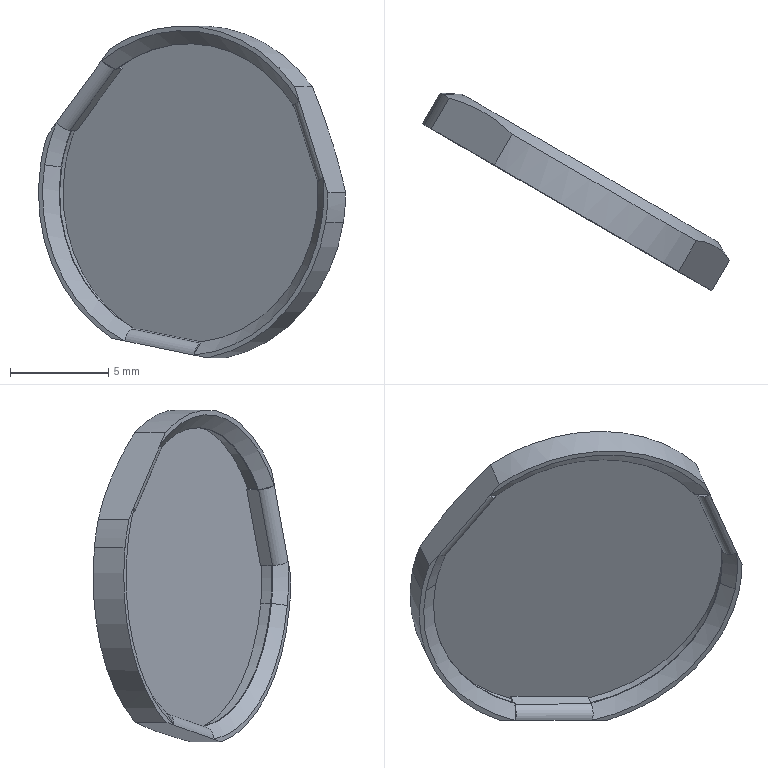Part | SolidWorks | features BaseBody 1 | 1 solid | 57 faces | box 15.622 x 10.059 x 16.879 mm | volume 251.42 mm3 | plane 32 | cylinder 18 | cone 7 | commonest cylinder face diameters 15.2 x5 15.6 x5 17 x5 1.2 x3